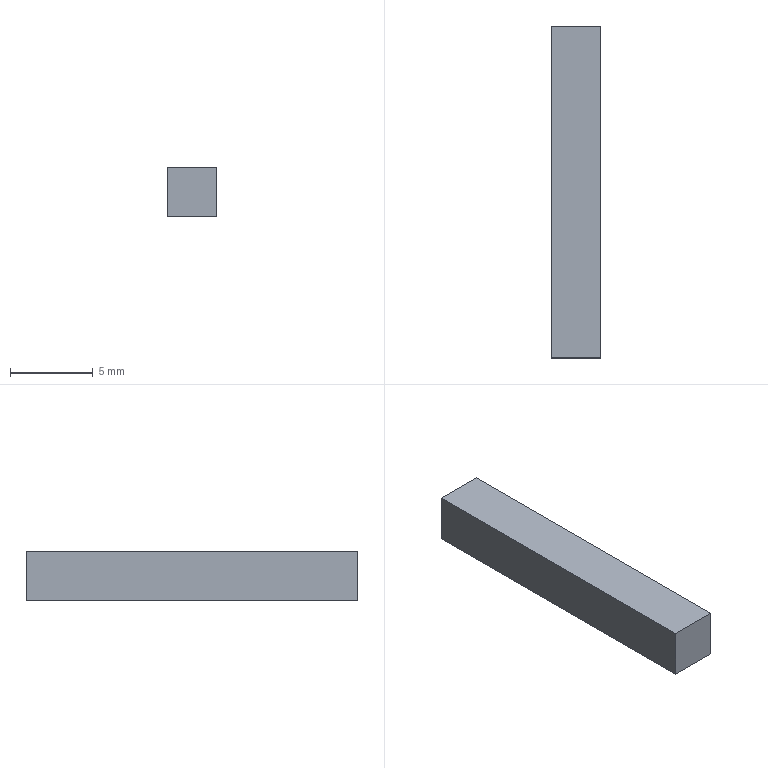Part | SolidWorks | features Extrusion 1 | 1 solid | 6 faces | box 3 x 20 x 3 mm | volume 180 mm3 | plane 6
STEP:
#1=CARTESIAN_POINT('',(1.5,0.,1.5));
#2=VERTEX_POINT('',#1);
#3=CARTESIAN_POINT('',(1.5,0.,-1.5));
#4=VERTEX_POINT('',#3);
#5=CARTESIAN_POINT('',(1.5,0.,1.5));
#6=DIRECTION('',(0.,0.,-1.));
#7=VECTOR('',#6,1000.);
#8=LINE('',#5,#7);
#9=EDGE_CURVE('',#2,#4,#8,.T.);
#10=ORIENTED_EDGE('',*,*,#9,.T.);
#11=CARTESIAN_POINT('',(1.5,20.,-1.5));
#12=VERTEX_POINT('',#11);
#13=CARTESIAN_POINT('',(1.5,20.,-1.5));
#14=DIRECTION('',(0.,-1.,0.));
#15=VECTOR('',#14,1000.);
#16=LINE('',#13,#15);
#17=EDGE_CURVE('',#12,#4,#16,.T.);
#18=ORIENTED_EDGE('',*,*,#17,.F.);
#19=CARTESIAN_POINT('',(1.5,20.,1.5));
#20=VERTEX_POINT('',#19);
#21=CARTESIAN_POINT('',(1.5,20.,1.5));
#22=DIRECTION('',(0.,0.,-1.));
#23=VECTOR('',#22,1000.);
#24=LINE('',#21,#23);
#25=EDGE_CURVE('',#20,#12,#24,.T.);
#26=ORIENTED_EDGE('',*,*,#25,.F.);
#27=CARTESIAN_POINT('',(1.5,20.,1.5));
#28=DIRECTION('',(0.,-1.,0.));
#29=VECTOR('',#28,1000.);
#30=LINE('',#27,#29);
#31=EDGE_CURVE('',#20,#2,#30,.T.);
#32=ORIENTED_EDGE('',*,*,#31,.T.);
#33=EDGE_LOOP('',(#10,#18,#26,#32));
#34=FACE_OUTER_BOUND('',#33,.T.);
#35=CARTESIAN_POINT('',(1.5,20.,1.5));
#36=DIRECTION('',(-1.,0.,0.));
#37=DIRECTION('',(0.,0.,1.));
#38=AXIS2_PLACEMENT_3D('',#35,#36,#37);
#39=PLANE('',#38);
#40=ADVANCED_FACE('',(#34),#39,.F.);
#41=CARTESIAN_POINT('',(-1.5,0.,-1.5));
#42=VERTEX_POINT('',#41);
#43=CARTESIAN_POINT('',(-1.5,0.,-1.5));
#44=DIRECTION('',(-1.,0.,0.));
#45=VECTOR('',#44,1000.);
#46=LINE('',#43,#45);
#47=EDGE_CURVE('',#4,#42,#46,.T.);
#48=ORIENTED_EDGE('',*,*,#47,.T.);
#49=CARTESIAN_POINT('',(-1.5,20.,-1.5));
#50=VERTEX_POINT('',#49);
#51=CARTESIAN_POINT('',(-1.5,20.,-1.5));
#52=DIRECTION('',(0.,-1.,0.));
#53=VECTOR('',#52,1000.);
#54=LINE('',#51,#53);
#55=EDGE_CURVE('',#50,#42,#54,.T.);
#56=ORIENTED_EDGE('',*,*,#55,.F.);
#57=CARTESIAN_POINT('',(-1.5,20.,-1.5));
#58=DIRECTION('',(-1.,0.,0.));
#59=VECTOR('',#58,1000.);
#60=LINE('',#57,#59);
#61=EDGE_CURVE('',#12,#50,#60,.T.);
#62=ORIENTED_EDGE('',*,*,#61,.F.);
#63=ORIENTED_EDGE('',*,*,#17,.T.);
#64=EDGE_LOOP('',(#48,#56,#62,#63));
#65=FACE_OUTER_BOUND('',#64,.T.);
#66=CARTESIAN_POINT('',(-1.5,20.,-1.5));
#67=DIRECTION('',(0.,0.,1.));
#68=DIRECTION('',(1.,0.,0.));
#69=AXIS2_PLACEMENT_3D('',#66,#67,#68);
#70=PLANE('',#69);
#71=ADVANCED_FACE('',(#65),#70,.F.);
#72=CARTESIAN_POINT('',(-1.5,0.,1.5));
#73=VERTEX_POINT('',#72);
#74=CARTESIAN_POINT('',(-1.5,0.,1.5));
#75=DIRECTION('',(0.,0.,1.));
#76=VECTOR('',#75,1000.);
#77=LINE('',#74,#76);
#78=EDGE_CURVE('',#42,#73,#77,.T.);
#79=ORIENTED_EDGE('',*,*,#78,.T.);
#80=CARTESIAN_POINT('',(-1.5,20.,1.5));
#81=VERTEX_POINT('',#80);
#82=CARTESIAN_POINT('',(-1.5,20.,1.5));
#83=DIRECTION('',(0.,-1.,0.));
#84=VECTOR('',#83,1000.);
#85=LINE('',#82,#84);
#86=EDGE_CURVE('',#81,#73,#85,.T.);
#87=ORIENTED_EDGE('',*,*,#86,.F.);
#88=CARTESIAN_POINT('',(-1.5,20.,1.5));
#89=DIRECTION('',(0.,0.,1.));
#90=VECTOR('',#89,1000.);
#91=LINE('',#88,#90);
#92=EDGE_CURVE('',#50,#81,#91,.T.);
#93=ORIENTED_EDGE('',*,*,#92,.F.);
#94=ORIENTED_EDGE('',*,*,#55,.T.);
#95=EDGE_LOOP('',(#79,#87,#93,#94));
#96=FACE_OUTER_BOUND('',#95,.T.);
#97=CARTESIAN_POINT('',(-1.5,20.,1.5));
#98=DIRECTION('',(1.,0.,0.));
#99=DIRECTION('',(0.,0.,-1.));
#100=AXIS2_PLACEMENT_3D('',#97,#98,#99);
#101=PLANE('',#100);
#102=ADVANCED_FACE('',(#96),#101,.F.);
#103=CARTESIAN_POINT('',(-1.5,0.,1.5));
#104=DIRECTION('',(1.,0.,0.));
#105=VECTOR('',#104,1000.);
#106=LINE('',#103,#105);
#107=EDGE_CURVE('',#73,#2,#106,.T.);
#108=ORIENTED_EDGE('',*,*,#107,.T.);
#109=ORIENTED_EDGE('',*,*,#31,.F.);
#110=CARTESIAN_POINT('',(-1.5,20.,1.5));
#111=DIRECTION('',(1.,0.,0.));
#112=VECTOR('',#111,1000.);
#113=LINE('',#110,#112);
#114=EDGE_CURVE('',#81,#20,#113,.T.);
#115=ORIENTED_EDGE('',*,*,#114,.F.);
#116=ORIENTED_EDGE('',*,*,#86,.T.);
#117=EDGE_LOOP('',(#108,#109,#115,#116));
#118=FACE_OUTER_BOUND('',#117,.T.);
#119=CARTESIAN_POINT('',(-1.5,20.,1.5));
#120=DIRECTION('',(0.,0.,-1.));
#121=DIRECTION('',(-1.,0.,0.));
#122=AXIS2_PLACEMENT_3D('',#119,#120,#121);
#123=PLANE('',#122);
#124=ADVANCED_FACE('',(#118),#123,.F.);
#125=ORIENTED_EDGE('',*,*,#25,.T.);
#126=ORIENTED_EDGE('',*,*,#61,.T.);
#127=ORIENTED_EDGE('',*,*,#92,.T.);
#128=ORIENTED_EDGE('',*,*,#114,.T.);
#129=EDGE_LOOP('',(#125,#126,#127,#128));
#130=FACE_OUTER_BOUND('',#129,.T.);
#131=CARTESIAN_POINT('',(0.,20.,0.));
#132=DIRECTION('',(0.,-1.,0.));
#133=DIRECTION('',(0.,0.,-1.));
#134=AXIS2_PLACEMENT_3D('',#131,#132,#133);
#135=PLANE('',#134);
#136=ADVANCED_FACE('',(#130),#135,.F.);
#137=ORIENTED_EDGE('',*,*,#9,.F.);
#138=ORIENTED_EDGE('',*,*,#107,.F.);
#139=ORIENTED_EDGE('',*,*,#78,.F.);
#140=ORIENTED_EDGE('',*,*,#47,.F.);
#141=EDGE_LOOP('',(#137,#138,#139,#140));
#142=FACE_OUTER_BOUND('',#141,.T.);
#143=CARTESIAN_POINT('',(0.,0.,0.));
#144=DIRECTION('',(0.,-1.,0.));
#145=DIRECTION('',(0.,0.,-1.));
#146=AXIS2_PLACEMENT_3D('',#143,#144,#145);
#147=PLANE('',#146);
#148=ADVANCED_FACE('',(#142),#147,.T.);
#149=CLOSED_SHELL('',(#40,#71,#102,#124,#136,#148));
#150=MANIFOLD_SOLID_BREP('',#149);
#151=CARTESIAN_POINT('',(0.,0.,0.));
#152=DIRECTION('',(0.,0.,1.));
#153=DIRECTION('',(1.,0.,0.));
#154=AXIS2_PLACEMENT_3D('',#151,#152,#153);
#155=(LENGTH_UNIT()NAMED_UNIT(*)SI_UNIT(.MILLI.,.METRE.));
#156=UNCERTAINTY_MEASURE_WITH_UNIT(LENGTH_MEASURE(0.00001),#155,'','');
#157=(NAMED_UNIT(*)PLANE_ANGLE_UNIT()SI_UNIT($,.RADIAN.));
#158=(NAMED_UNIT(*)SI_UNIT($,.STERADIAN.)SOLID_ANGLE_UNIT());
#159=(GEOMETRIC_REPRESENTATION_CONTEXT(3)GLOBAL_UNCERTAINTY_ASSIGNED_CONTEXT((#156))GLOBAL_UNIT_ASSIGNED_CONTEXT((#155,#157,#158))REPRESENTATION_CONTEXT('',''));
#160=ADVANCED_BREP_SHAPE_REPRESENTATION('',(#150,#154),#159);